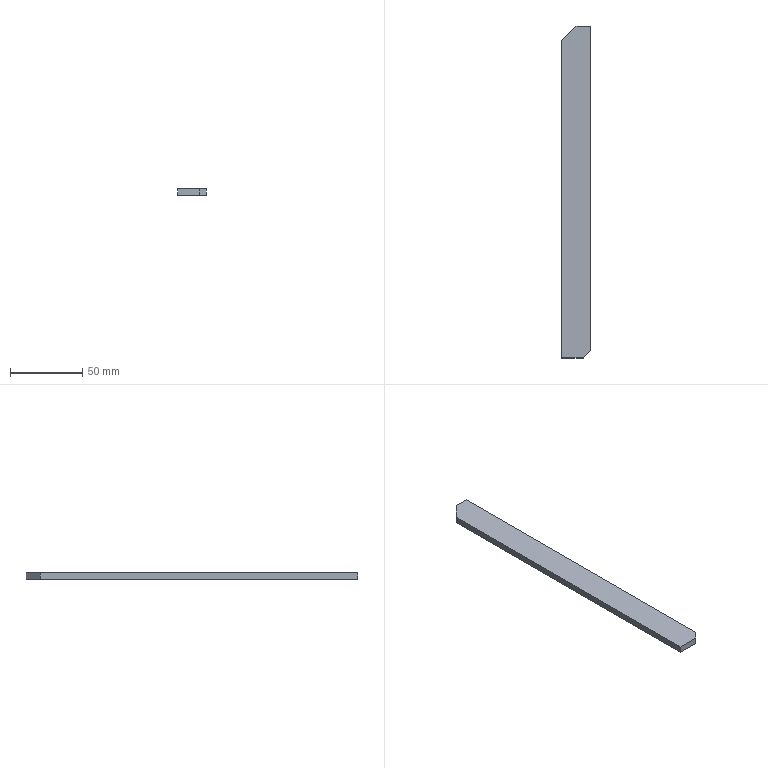Part | SolidWorks | features FlatPattern 1, SMBaseFlange 1, SheetMetal 1 | 1 solid | 8 faces | box 20 x 230 x 4.5 mm | volume 20419 mm3 | plane 8
STEP:
#1=CARTESIAN_POINT('',(-10.,-115.,0.));
#2=VERTEX_POINT('',#1);
#3=CARTESIAN_POINT('',(5.,-115.,0.));
#4=VERTEX_POINT('',#3);
#5=CARTESIAN_POINT('',(-10.,-115.,0.));
#6=DIRECTION('',(1.,0.,0.));
#7=VECTOR('',#6,1000.);
#8=LINE('',#5,#7);
#9=EDGE_CURVE('',#2,#4,#8,.T.);
#10=ORIENTED_EDGE('',*,*,#9,.F.);
#11=CARTESIAN_POINT('',(-10.,-115.,-4.5));
#12=VERTEX_POINT('',#11);
#13=CARTESIAN_POINT('',(-10.,-115.,-4.5));
#14=DIRECTION('',(0.,0.,1.));
#15=VECTOR('',#14,1000.);
#16=LINE('',#13,#15);
#17=EDGE_CURVE('',#12,#2,#16,.T.);
#18=ORIENTED_EDGE('',*,*,#17,.F.);
#19=CARTESIAN_POINT('',(5.,-115.,-4.5));
#20=VERTEX_POINT('',#19);
#21=CARTESIAN_POINT('',(-10.,-115.,-4.5));
#22=DIRECTION('',(1.,0.,0.));
#23=VECTOR('',#22,1000.);
#24=LINE('',#21,#23);
#25=EDGE_CURVE('',#12,#20,#24,.T.);
#26=ORIENTED_EDGE('',*,*,#25,.T.);
#27=CARTESIAN_POINT('',(5.,-115.,-4.5));
#28=DIRECTION('',(0.,0.,1.));
#29=VECTOR('',#28,1000.);
#30=LINE('',#27,#29);
#31=EDGE_CURVE('',#20,#4,#30,.T.);
#32=ORIENTED_EDGE('',*,*,#31,.T.);
#33=EDGE_LOOP('',(#10,#18,#26,#32));
#34=FACE_OUTER_BOUND('',#33,.T.);
#35=CARTESIAN_POINT('',(-10.,-115.,-4.5));
#36=DIRECTION('',(0.,-1.,0.));
#37=DIRECTION('',(0.,0.,-1.));
#38=AXIS2_PLACEMENT_3D('',#35,#36,#37);
#39=PLANE('',#38);
#40=ADVANCED_FACE('',(#34),#39,.T.);
#41=CARTESIAN_POINT('',(-10.,105.,0.));
#42=VERTEX_POINT('',#41);
#43=CARTESIAN_POINT('',(-10.,105.,0.));
#44=DIRECTION('',(0.,-1.,0.));
#45=VECTOR('',#44,1000.);
#46=LINE('',#43,#45);
#47=EDGE_CURVE('',#42,#2,#46,.T.);
#48=ORIENTED_EDGE('',*,*,#47,.F.);
#49=CARTESIAN_POINT('',(-10.,105.,-4.5));
#50=VERTEX_POINT('',#49);
#51=CARTESIAN_POINT('',(-10.,105.,-4.5));
#52=DIRECTION('',(0.,0.,1.));
#53=VECTOR('',#52,1000.);
#54=LINE('',#51,#53);
#55=EDGE_CURVE('',#50,#42,#54,.T.);
#56=ORIENTED_EDGE('',*,*,#55,.F.);
#57=CARTESIAN_POINT('',(-10.,105.,-4.5));
#58=DIRECTION('',(0.,-1.,0.));
#59=VECTOR('',#58,1000.);
#60=LINE('',#57,#59);
#61=EDGE_CURVE('',#50,#12,#60,.T.);
#62=ORIENTED_EDGE('',*,*,#61,.T.);
#63=ORIENTED_EDGE('',*,*,#17,.T.);
#64=EDGE_LOOP('',(#48,#56,#62,#63));
#65=FACE_OUTER_BOUND('',#64,.T.);
#66=CARTESIAN_POINT('',(-10.,105.,-4.5));
#67=DIRECTION('',(-1.,0.,0.));
#68=DIRECTION('',(0.,-1.,0.));
#69=AXIS2_PLACEMENT_3D('',#66,#67,#68);
#70=PLANE('',#69);
#71=ADVANCED_FACE('',(#65),#70,.T.);
#72=CARTESIAN_POINT('',(0.,115.,0.));
#73=VERTEX_POINT('',#72);
#74=CARTESIAN_POINT('',(-10.,105.,0.));
#75=DIRECTION('',(-0.7071,-0.7071,0.));
#76=VECTOR('',#75,1000.);
#77=LINE('',#74,#76);
#78=EDGE_CURVE('',#73,#42,#77,.T.);
#79=ORIENTED_EDGE('',*,*,#78,.F.);
#80=CARTESIAN_POINT('',(0.,115.,-4.5));
#81=VERTEX_POINT('',#80);
#82=CARTESIAN_POINT('',(0.,115.,-4.5));
#83=DIRECTION('',(0.,0.,1.));
#84=VECTOR('',#83,1000.);
#85=LINE('',#82,#84);
#86=EDGE_CURVE('',#81,#73,#85,.T.);
#87=ORIENTED_EDGE('',*,*,#86,.F.);
#88=CARTESIAN_POINT('',(-10.,105.,-4.5));
#89=DIRECTION('',(-0.7071,-0.7071,0.));
#90=VECTOR('',#89,1000.);
#91=LINE('',#88,#90);
#92=EDGE_CURVE('',#81,#50,#91,.T.);
#93=ORIENTED_EDGE('',*,*,#92,.T.);
#94=ORIENTED_EDGE('',*,*,#55,.T.);
#95=EDGE_LOOP('',(#79,#87,#93,#94));
#96=FACE_OUTER_BOUND('',#95,.T.);
#97=CARTESIAN_POINT('',(-10.,105.,-4.5));
#98=DIRECTION('',(-0.7071,0.7071,0.));
#99=DIRECTION('',(-0.7071,-0.7071,0.));
#100=AXIS2_PLACEMENT_3D('',#97,#98,#99);
#101=PLANE('',#100);
#102=ADVANCED_FACE('',(#96),#101,.T.);
#103=CARTESIAN_POINT('',(10.,115.,0.));
#104=VERTEX_POINT('',#103);
#105=CARTESIAN_POINT('',(0.,115.,0.));
#106=DIRECTION('',(-1.,0.,0.));
#107=VECTOR('',#106,1000.);
#108=LINE('',#105,#107);
#109=EDGE_CURVE('',#104,#73,#108,.T.);
#110=ORIENTED_EDGE('',*,*,#109,.F.);
#111=CARTESIAN_POINT('',(10.,115.,-4.5));
#112=VERTEX_POINT('',#111);
#113=CARTESIAN_POINT('',(10.,115.,-4.5));
#114=DIRECTION('',(0.,0.,1.));
#115=VECTOR('',#114,1000.);
#116=LINE('',#113,#115);
#117=EDGE_CURVE('',#112,#104,#116,.T.);
#118=ORIENTED_EDGE('',*,*,#117,.F.);
#119=CARTESIAN_POINT('',(0.,115.,-4.5));
#120=DIRECTION('',(-1.,0.,0.));
#121=VECTOR('',#120,1000.);
#122=LINE('',#119,#121);
#123=EDGE_CURVE('',#112,#81,#122,.T.);
#124=ORIENTED_EDGE('',*,*,#123,.T.);
#125=ORIENTED_EDGE('',*,*,#86,.T.);
#126=EDGE_LOOP('',(#110,#118,#124,#125));
#127=FACE_OUTER_BOUND('',#126,.T.);
#128=CARTESIAN_POINT('',(0.,115.,-4.5));
#129=DIRECTION('',(0.,1.,0.));
#130=DIRECTION('',(0.,0.,1.));
#131=AXIS2_PLACEMENT_3D('',#128,#129,#130);
#132=PLANE('',#131);
#133=ADVANCED_FACE('',(#127),#132,.T.);
#134=CARTESIAN_POINT('',(10.,-110.,0.));
#135=VERTEX_POINT('',#134);
#136=CARTESIAN_POINT('',(10.,115.,0.));
#137=DIRECTION('',(0.,1.,0.));
#138=VECTOR('',#137,1000.);
#139=LINE('',#136,#138);
#140=EDGE_CURVE('',#135,#104,#139,.T.);
#141=ORIENTED_EDGE('',*,*,#140,.F.);
#142=CARTESIAN_POINT('',(10.,-110.,-4.5));
#143=VERTEX_POINT('',#142);
#144=CARTESIAN_POINT('',(10.,-110.,-4.5));
#145=DIRECTION('',(0.,0.,1.));
#146=VECTOR('',#145,1000.);
#147=LINE('',#144,#146);
#148=EDGE_CURVE('',#143,#135,#147,.T.);
#149=ORIENTED_EDGE('',*,*,#148,.F.);
#150=CARTESIAN_POINT('',(10.,115.,-4.5));
#151=DIRECTION('',(0.,1.,0.));
#152=VECTOR('',#151,1000.);
#153=LINE('',#150,#152);
#154=EDGE_CURVE('',#143,#112,#153,.T.);
#155=ORIENTED_EDGE('',*,*,#154,.T.);
#156=ORIENTED_EDGE('',*,*,#117,.T.);
#157=EDGE_LOOP('',(#141,#149,#155,#156));
#158=FACE_OUTER_BOUND('',#157,.T.);
#159=CARTESIAN_POINT('',(10.,115.,-4.5));
#160=DIRECTION('',(1.,0.,0.));
#161=DIRECTION('',(0.,1.,0.));
#162=AXIS2_PLACEMENT_3D('',#159,#160,#161);
#163=PLANE('',#162);
#164=ADVANCED_FACE('',(#158),#163,.T.);
#165=CARTESIAN_POINT('',(5.,-115.,0.));
#166=DIRECTION('',(0.7071,0.7071,0.));
#167=VECTOR('',#166,1000.);
#168=LINE('',#165,#167);
#169=EDGE_CURVE('',#4,#135,#168,.T.);
#170=ORIENTED_EDGE('',*,*,#169,.F.);
#171=ORIENTED_EDGE('',*,*,#31,.F.);
#172=CARTESIAN_POINT('',(5.,-115.,-4.5));
#173=DIRECTION('',(0.7071,0.7071,0.));
#174=VECTOR('',#173,1000.);
#175=LINE('',#172,#174);
#176=EDGE_CURVE('',#20,#143,#175,.T.);
#177=ORIENTED_EDGE('',*,*,#176,.T.);
#178=ORIENTED_EDGE('',*,*,#148,.T.);
#179=EDGE_LOOP('',(#170,#171,#177,#178));
#180=FACE_OUTER_BOUND('',#179,.T.);
#181=CARTESIAN_POINT('',(5.,-115.,-4.5));
#182=DIRECTION('',(0.7071,-0.7071,0.));
#183=DIRECTION('',(0.7071,0.7071,0.));
#184=AXIS2_PLACEMENT_3D('',#181,#182,#183);
#185=PLANE('',#184);
#186=ADVANCED_FACE('',(#180),#185,.T.);
#187=ORIENTED_EDGE('',*,*,#25,.F.);
#188=ORIENTED_EDGE('',*,*,#61,.F.);
#189=ORIENTED_EDGE('',*,*,#92,.F.);
#190=ORIENTED_EDGE('',*,*,#123,.F.);
#191=ORIENTED_EDGE('',*,*,#154,.F.);
#192=ORIENTED_EDGE('',*,*,#176,.F.);
#193=EDGE_LOOP('',(#187,#188,#189,#190,#191,#192));
#194=FACE_OUTER_BOUND('',#193,.T.);
#195=CARTESIAN_POINT('',(0.,0.,-4.5));
#196=DIRECTION('',(0.,0.,-1.));
#197=DIRECTION('',(-1.,0.,0.));
#198=AXIS2_PLACEMENT_3D('',#195,#196,#197);
#199=PLANE('',#198);
#200=ADVANCED_FACE('',(#194),#199,.T.);
#201=ORIENTED_EDGE('',*,*,#9,.T.);
#202=ORIENTED_EDGE('',*,*,#169,.T.);
#203=ORIENTED_EDGE('',*,*,#140,.T.);
#204=ORIENTED_EDGE('',*,*,#109,.T.);
#205=ORIENTED_EDGE('',*,*,#78,.T.);
#206=ORIENTED_EDGE('',*,*,#47,.T.);
#207=EDGE_LOOP('',(#201,#202,#203,#204,#205,#206));
#208=FACE_OUTER_BOUND('',#207,.T.);
#209=CARTESIAN_POINT('',(0.,0.,0.));
#210=DIRECTION('',(0.,0.,-1.));
#211=DIRECTION('',(-1.,0.,0.));
#212=AXIS2_PLACEMENT_3D('',#209,#210,#211);
#213=PLANE('',#212);
#214=ADVANCED_FACE('',(#208),#213,.F.);
#215=CLOSED_SHELL('',(#40,#71,#102,#133,#164,#186,#200,#214));
#216=MANIFOLD_SOLID_BREP('',#215);
#217=CARTESIAN_POINT('',(0.,0.,0.));
#218=DIRECTION('',(0.,0.,1.));
#219=DIRECTION('',(1.,0.,0.));
#220=AXIS2_PLACEMENT_3D('',#217,#218,#219);
#221=(LENGTH_UNIT()NAMED_UNIT(*)SI_UNIT(.MILLI.,.METRE.));
#222=UNCERTAINTY_MEASURE_WITH_UNIT(LENGTH_MEASURE(0.00001),#221,'','');
#223=(NAMED_UNIT(*)PLANE_ANGLE_UNIT()SI_UNIT($,.RADIAN.));
#224=(NAMED_UNIT(*)SI_UNIT($,.STERADIAN.)SOLID_ANGLE_UNIT());
#225=(GEOMETRIC_REPRESENTATION_CONTEXT(3)GLOBAL_UNCERTAINTY_ASSIGNED_CONTEXT((#222))GLOBAL_UNIT_ASSIGNED_CONTEXT((#221,#223,#224))REPRESENTATION_CONTEXT('',''));
#226=ADVANCED_BREP_SHAPE_REPRESENTATION('',(#216,#220),#225);